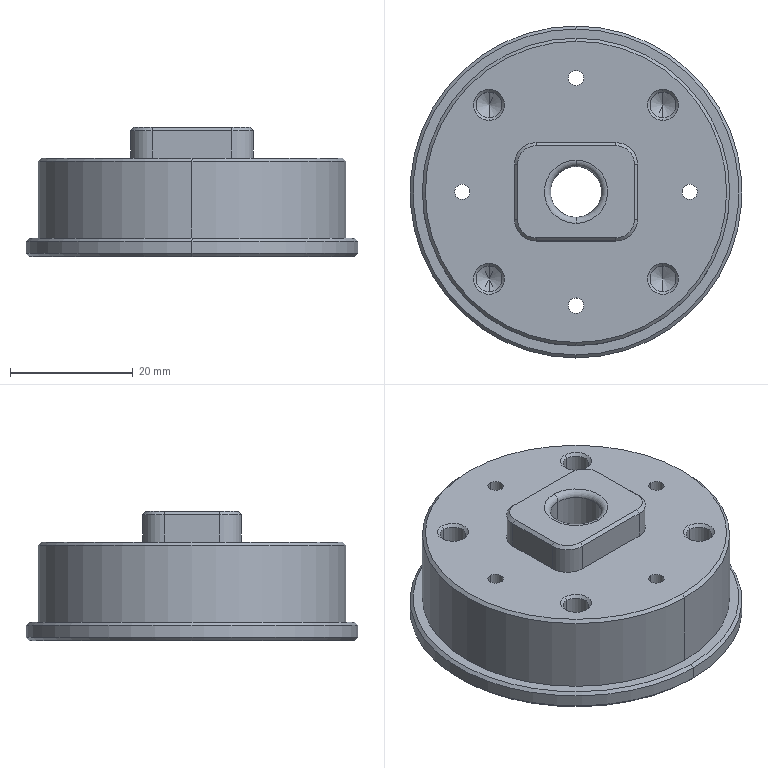NC program | NX | posted with a generic post | part box 54 x 54 x 21 mm
Lines 246 to 1139 of 9691:
(FLOOR_WALL_1_COPY_1 , TOOL : D4)
N478 T11 M6
N480 G54
N482 G17 G0 G90 X7.027 Y6.145 S9500 M3
N484 G43 Z30. H11
N486 Z1.5
N488 G94 G1 X7.252 Y5.92 Z1.483 F2200.
N490 X8.29 Y4.349 Z1.385
N492 X8.993 Y2.602 Z1.286
N494 X9.332 Y0.749 Z1.187
N496 Y-0.749 Z1.109
N498 X8.993 Y-2.602 Z1.01
N500 X8.29 Y-4.349 Z0.911
N502 X7.252 Y-5.92 Z0.813
N504 X5.92 Y-7.252 Z0.714
N506 X4.349 Y-8.29 Z0.615
N508 X2.602 Y-8.993 Z0.516
N510 X0.749 Y-9.332 Z0.418
N512 X-0.749 Z0.339
N514 X-2.602 Y-8.993 Z0.241
N516 X-4.349 Y-8.29 Z0.142
N518 X-5.92 Y-7.252 Z0.043
N520 X-7.252 Y-5.92 Z-0.056
N522 X-8.29 Y-4.349 Z-0.154
N524 X-8.993 Y-2.602 Z-0.253
N526 X-9.332 Y-0.749 Z-0.352
N528 Y0. Z-0.391
N530 G2 X0. Y9.332 R9.332
N532 X-9.332 Y0. R-9.332
N534 G1 X-9.9
N536 G3 X-9.895 Y-0.317 R9.9
N538 G2 X-11.188 Y-4.634 R7.1
N540 X-7.221 Y-6.773 R7.1
N542 G3 X-6.773 Y-7.221 R9.9
N544 G2 X-4.634 Y-11.188 R7.1
N546 X-0.317 Y-9.895 R7.1
N548 G3 X0.317 Y-9.895 R9.9
N550 G2 X4.634 Y-11.188 R7.1
N552 X6.773 Y-7.221 R7.1
N554 G3 X7.221 Y-6.773 R9.9
N556 G2 X11.188 Y-4.634 R7.1
N558 X9.895 Y-0.317 R7.1
N560 G3 X9.895 Y0.317 R9.9
N562 G2 X11.188 Y4.634 R7.1
N564 X7.221 Y6.773 R7.1
N566 G3 X6.773 Y7.221 R9.9
N568 G2 X4.634 Y11.188 R7.1
N570 X0.317 Y9.895 R7.1
N572 G3 X-0.317 Y9.895 R9.9
N574 G2 X-4.634 Y11.188 R7.1
N576 X-6.773 Y7.221 R7.1
N578 G3 X-7.221 Y6.773 R9.9
N580 G2 X-11.188 Y4.634 R7.1
N582 X-9.895 Y0.317 R7.1
N584 G3 X-9.9 Y0. R9.9
N586 G1 X-11.9
N588 G3 X-11.894 Y-0.381 R11.9
N590 G2 X-15.04 Y-5.255 R5.1
N592 G1 X-18.822 Y-6.822
N594 G3 X-19.309 Y-7.998 R0.9
N596 X-18.133 Y-8.485 R0.9
N598 G1 X-14.351 Y-6.918
N600 G2 X-8.679 Y-8.141 R5.1
N602 G3 X-8.141 Y-8.679 R11.9
N604 G2 X-6.918 Y-14.351 R5.1
N606 G1 X-8.485 Y-18.133
N608 G3 X-7.998 Y-19.309 R0.9
N610 X-6.822 Y-18.822 R0.9
N612 G1 X-5.255 Y-15.04
N614 G2 X-0.381 Y-11.894 R5.1
N616 G3 X0.381 Y-11.894 R11.9
N618 G2 X5.255 Y-15.04 R5.1
N620 G1 X6.822 Y-18.822
N622 G3 X7.998 Y-19.309 R0.9
N624 X8.485 Y-18.133 R0.9
N626 G1 X6.918 Y-14.351
N628 G2 X8.141 Y-8.679 R5.1
N630 G3 X8.679 Y-8.141 R11.9
N632 G2 X14.351 Y-6.918 R5.1
N634 G1 X18.133 Y-8.485
N636 G3 X19.309 Y-7.998 R0.9
N638 X18.822 Y-6.822 R0.9
N640 G1 X15.04 Y-5.255
N642 G2 X11.894 Y-0.381 R5.1
N644 G3 X11.894 Y0.381 R11.9
N646 G2 X15.04 Y5.255 R5.1
N648 G1 X18.822 Y6.822
N650 G3 X19.309 Y7.998 R0.9
N652 X18.133 Y8.485 R0.9
N654 G1 X14.351 Y6.918
N656 G2 X8.679 Y8.141 R5.1
N658 G3 X8.141 Y8.679 R11.9
N660 G2 X6.918 Y14.351 R5.1
N662 G1 X8.485 Y18.133
N664 G3 X7.998 Y19.309 R0.9
N666 X6.822 Y18.822 R0.9
N668 G1 X5.255 Y15.04
N670 G2 X0.381 Y11.894 R5.1
N672 G3 X-0.381 Y11.894 R11.9
N674 G2 X-5.255 Y15.04 R5.1
N676 G1 X-6.822 Y18.822
N678 G3 X-7.998 Y19.309 R0.9
N680 X-8.485 Y18.133 R0.9
N682 G1 X-6.918 Y14.351
N684 G2 X-8.141 Y8.679 R5.1
N686 G3 X-8.679 Y8.141 R11.9
N688 G2 X-14.351 Y6.918 R5.1
N690 G1 X-18.133 Y8.485
N692 G3 X-19.309 Y7.998 R0.9
N694 X-18.822 Y6.822 R0.9
N696 G1 X-15.04 Y5.255
N698 G2 X-11.894 Y0.381 R5.1
N700 G3 X-11.9 Y0. R11.9
N702 G1 Z1.109
N704 G0 Z30.
N706 X7.027 Y6.145
N708 Z1.109
N710 G1 X7.252 Y5.92 Z1.092
N712 X8.29 Y4.349 Z0.994
N714 X8.993 Y2.602 Z0.895
N716 X9.332 Y0.749 Z0.796
N718 Y-0.749 Z0.718
N720 X8.993 Y-2.602 Z0.619
N722 X8.29 Y-4.349 Z0.52
N724 X7.252 Y-5.92 Z0.422
N726 X5.92 Y-7.252 Z0.323
N728 X4.349 Y-8.29 Z0.224
N730 X2.602 Y-8.993 Z0.126
N732 X0.749 Y-9.332 Z0.027
N734 X-0.749 Z-0.052
N736 X-2.602 Y-8.993 Z-0.15
N738 X-4.349 Y-8.29 Z-0.249
N740 X-5.92 Y-7.252 Z-0.348
N742 X-7.252 Y-5.92 Z-0.446
N744 X-8.29 Y-4.349 Z-0.545
N746 X-8.993 Y-2.602 Z-0.644
N748 X-9.332 Y-0.749 Z-0.743
N750 Y0. Z-0.782
N752 G2 X0. Y9.332 R9.332
N754 X-9.332 Y0. R-9.332
N756 G1 X-9.9
N758 G3 X-9.895 Y-0.317 R9.9
N760 G2 X-11.188 Y-4.634 R7.1
N762 X-7.221 Y-6.773 R7.1
N764 G3 X-6.773 Y-7.221 R9.9
N766 G2 X-4.634 Y-11.188 R7.1
N768 X-0.317 Y-9.895 R7.1
N770 G3 X0.317 Y-9.895 R9.9
N772 G2 X4.634 Y-11.188 R7.1
N774 X6.773 Y-7.221 R7.1
N776 G3 X7.221 Y-6.773 R9.9
N778 G2 X11.188 Y-4.634 R7.1
N780 X9.895 Y-0.317 R7.1
N782 G3 X9.895 Y0.317 R9.9
N784 G2 X11.188 Y4.634 R7.1
N786 X7.221 Y6.773 R7.1
N788 G3 X6.773 Y7.221 R9.9
N790 G2 X4.634 Y11.188 R7.1
N792 X0.317 Y9.895 R7.1
N794 G3 X-0.317 Y9.895 R9.9
N796 G2 X-4.634 Y11.188 R7.1
N798 X-6.773 Y7.221 R7.1
N800 G3 X-7.221 Y6.773 R9.9
N802 G2 X-11.188 Y4.634 R7.1
N804 X-9.895 Y0.317 R7.1
N806 G3 X-9.9 Y0. R9.9
N808 G1 X-11.9
N810 G3 X-11.894 Y-0.381 R11.9
N812 G2 X-15.04 Y-5.255 R5.1
N814 G1 X-18.822 Y-6.822
N816 G3 X-19.309 Y-7.998 R0.9
N818 X-18.133 Y-8.485 R0.9
N820 G1 X-14.351 Y-6.918
N822 G2 X-8.679 Y-8.141 R5.1
N824 G3 X-8.141 Y-8.679 R11.9
N826 G2 X-6.918 Y-14.351 R5.1
N828 G1 X-8.485 Y-18.133
N830 G3 X-7.998 Y-19.309 R0.9
N832 X-6.822 Y-18.822 R0.9
N834 G1 X-5.255 Y-15.04
N836 G2 X-0.381 Y-11.894 R5.1
N838 G3 X0.381 Y-11.894 R11.9
N840 G2 X5.255 Y-15.04 R5.1
N842 G1 X6.822 Y-18.822
N844 G3 X7.998 Y-19.309 R0.9
N846 X8.485 Y-18.133 R0.9
N848 G1 X6.918 Y-14.351
N850 G2 X8.141 Y-8.679 R5.1
N852 G3 X8.679 Y-8.141 R11.9
N854 G2 X14.351 Y-6.918 R5.1
N856 G1 X18.133 Y-8.485
N858 G3 X19.309 Y-7.998 R0.9
N860 X18.822 Y-6.822 R0.9
N862 G1 X15.04 Y-5.255
N864 G2 X11.894 Y-0.381 R5.1
N866 G3 X11.894 Y0.381 R11.9
N868 G2 X15.04 Y5.255 R5.1
N870 G1 X18.822 Y6.822
N872 G3 X19.309 Y7.998 R0.9
N874 X18.133 Y8.485 R0.9
N876 G1 X14.351 Y6.918
N878 G2 X8.679 Y8.141 R5.1
N880 G3 X8.141 Y8.679 R11.9
N882 G2 X6.918 Y14.351 R5.1
N884 G1 X8.485 Y18.133
N886 G3 X7.998 Y19.309 R0.9
N888 X6.822 Y18.822 R0.9
N890 G1 X5.255 Y15.04
N892 G2 X0.381 Y11.894 R5.1
N894 G3 X-0.381 Y11.894 R11.9
N896 G2 X-5.255 Y15.04 R5.1
N898 G1 X-6.822 Y18.822
N900 G3 X-7.998 Y19.309 R0.9
N902 X-8.485 Y18.133 R0.9
N904 G1 X-6.918 Y14.351
N906 G2 X-8.141 Y8.679 R5.1
N908 G3 X-8.679 Y8.141 R11.9
N910 G2 X-14.351 Y6.918 R5.1
N912 G1 X-18.133 Y8.485
N914 G3 X-19.309 Y7.998 R0.9
N916 X-18.822 Y6.822 R0.9
N918 G1 X-15.04 Y5.255
N920 G2 X-11.894 Y0.381 R5.1
N922 G3 X-11.9 Y0. R11.9
N924 G1 Z0.718
N926 G0 Z30.
N928 X7.027 Y6.145
N930 Z0.718
N932 G1 X7.252 Y5.92 Z0.702
N934 X8.29 Y4.349 Z0.603
N936 X8.993 Y2.602 Z0.504
N938 X9.332 Y0.749 Z0.405
N940 Y-0.749 Z0.327
N942 X8.993 Y-2.602 Z0.228
N944 X8.29 Y-4.349 Z0.129
N946 X7.252 Y-5.92 Z0.031
N948 X5.92 Y-7.252 Z-0.068
N950 X4.349 Y-8.29 Z-0.167
N952 X2.602 Y-8.993 Z-0.265
N954 X0.749 Y-9.332 Z-0.364
N956 X-0.749 Z-0.443
N958 X-2.602 Y-8.993 Z-0.541
N960 X-4.349 Y-8.29 Z-0.64
N962 X-5.92 Y-7.252 Z-0.739
N964 X-7.252 Y-5.92 Z-0.837
N966 X-8.29 Y-4.349 Z-0.936
N968 X-8.993 Y-2.602 Z-1.035
N970 X-9.332 Y-0.749 Z-1.133
N972 Y0. Z-1.173
N974 G2 X0. Y9.332 R9.332
N976 X-9.332 Y0. R-9.332
N978 G1 X-9.9
N980 G3 X-9.895 Y-0.317 R9.9
N982 G2 X-11.188 Y-4.634 R7.1
N984 X-7.221 Y-6.773 R7.1
N986 G3 X-6.773 Y-7.221 R9.9
N988 G2 X-4.634 Y-11.188 R7.1
N990 X-0.317 Y-9.895 R7.1
N992 G3 X0.317 Y-9.895 R9.9
N994 G2 X4.634 Y-11.188 R7.1
N996 X6.773 Y-7.221 R7.1
N998 G3 X7.221 Y-6.773 R9.9
N1000 G2 X11.188 Y-4.634 R7.1
N1002 X9.895 Y-0.317 R7.1
N1004 G3 X9.895 Y0.317 R9.9
N1006 G2 X11.188 Y4.634 R7.1
N1008 X7.221 Y6.773 R7.1
N1010 G3 X6.773 Y7.221 R9.9
N1012 G2 X4.634 Y11.188 R7.1
N1014 X0.317 Y9.895 R7.1
N1016 G3 X-0.317 Y9.895 R9.9
N1018 G2 X-4.634 Y11.188 R7.1
N1020 X-6.773 Y7.221 R7.1
N1022 G3 X-7.221 Y6.773 R9.9
N1024 G2 X-11.188 Y4.634 R7.1
N1026 X-9.895 Y0.317 R7.1
N1028 G3 X-9.9 Y0. R9.9
N1030 G1 X-11.9
N1032 G3 X-11.894 Y-0.381 R11.9
N1034 G2 X-15.04 Y-5.255 R5.1
N1036 G1 X-18.822 Y-6.822
N1038 G3 X-19.309 Y-7.998 R0.9
N1040 X-18.133 Y-8.485 R0.9
N1042 G1 X-14.351 Y-6.918
N1044 G2 X-8.679 Y-8.141 R5.1
N1046 G3 X-8.141 Y-8.679 R11.9
N1048 G2 X-6.918 Y-14.351 R5.1
N1050 G1 X-8.485 Y-18.133
N1052 G3 X-7.998 Y-19.309 R0.9
N1054 X-6.822 Y-18.822 R0.9
N1056 G1 X-5.255 Y-15.04
N1058 G2 X-0.381 Y-11.894 R5.1
N1060 G3 X0.381 Y-11.894 R11.9
N1062 G2 X5.255 Y-15.04 R5.1
N1064 G1 X6.822 Y-18.822
N1066 G3 X7.998 Y-19.309 R0.9
N1068 X8.485 Y-18.133 R0.9
N1070 G1 X6.918 Y-14.351
N1072 G2 X8.141 Y-8.679 R5.1
N1074 G3 X8.679 Y-8.141 R11.9
N1076 G2 X14.351 Y-6.918 R5.1
N1078 G1 X18.133 Y-8.485
N1080 G3 X19.309 Y-7.998 R0.9
N1082 X18.822 Y-6.822 R0.9
N1084 G1 X15.04 Y-5.255
N1086 G2 X11.894 Y-0.381 R5.1
N1088 G3 X11.894 Y0.381 R11.9
N1090 G2 X15.04 Y5.255 R5.1
N1092 G1 X18.822 Y6.822
N1094 G3 X19.309 Y7.998 R0.9
N1096 X18.133 Y8.485 R0.9
N1098 G1 X14.351 Y6.918
N1100 G2 X8.679 Y8.141 R5.1
N1102 G3 X8.141 Y8.679 R11.9
N1104 G2 X6.918 Y14.351 R5.1
N1106 G1 X8.485 Y18.133
N1108 G3 X7.998 Y19.309 R0.9
N1110 X6.822 Y18.822 R0.9
N1112 G1 X5.255 Y15.04
N1114 G2 X0.381 Y11.894 R5.1
N1116 G3 X-0.381 Y11.894 R11.9
N1118 G2 X-5.255 Y15.04 R5.1
N1120 G1 X-6.822 Y18.822
N1122 G3 X-7.998 Y19.309 R0.9
N1124 X-8.485 Y18.133 R0.9
N1126 G1 X-6.918 Y14.351
N1128 G2 X-8.141 Y8.679 R5.1
N1130 G3 X-8.679 Y8.141 R11.9
N1132 G2 X-14.351 Y6.918 R5.1
N1134 G1 X-18.133 Y8.485
N1136 G3 X-19.309 Y7.998 R0.9
N1138 X-18.822 Y6.822 R0.9
N1140 G1 X-15.04 Y5.255
N1142 G2 X-11.894 Y0.381 R5.1
N1144 G3 X-11.9 Y0. R11.9
N1146 G1 Z0.327
N1148 G0 Z30.
N1150 X7.027 Y6.145
N1152 Z0.327
N1154 G1 X7.252 Y5.92 Z0.311
N1156 X8.29 Y4.349 Z0.212
N1158 X8.993 Y2.602 Z0.113
N1160 X9.332 Y0.749 Z0.014
N1162 Y-0.749 Z-0.064
N1164 X8.993 Y-2.602 Z-0.163
N1166 X8.29 Y-4.349 Z-0.261
N1168 X7.252 Y-5.92 Z-0.36
N1170 X5.92 Y-7.252 Z-0.459
N1172 X4.349 Y-8.29 Z-0.558
N1174 X2.602 Y-8.993 Z-0.656
N1176 X0.749 Y-9.332 Z-0.755
N1178 X-0.749 Z-0.833
N1180 X-2.602 Y-8.993 Z-0.932
N1182 X-4.349 Y-8.29 Z-1.031
N1184 X-5.92 Y-7.252 Z-1.13
N1186 X-7.252 Y-5.92 Z-1.228
N1188 X-8.29 Y-4.349 Z-1.327
N1190 X-8.993 Y-2.602 Z-1.426
N1192 X-9.332 Y-0.749 Z-1.524
N1194 Y0. Z-1.564
N1196 G2 X0. Y9.332 R9.332
N1198 X-9.332 Y0. R-9.332
N1200 G1 X-9.9
N1202 G3 X-9.895 Y-0.317 R9.9
N1204 G2 X-11.188 Y-4.634 R7.1
N1206 X-7.221 Y-6.773 R7.1
N1208 G3 X-6.773 Y-7.221 R9.9
N1210 G2 X-4.634 Y-11.188 R7.1
N1212 X-0.317 Y-9.895 R7.1
N1214 G3 X0.317 Y-9.895 R9.9
N1216 G2 X4.634 Y-11.188 R7.1
N1218 X6.773 Y-7.221 R7.1
N1220 G3 X7.221 Y-6.773 R9.9
N1222 G2 X11.188 Y-4.634 R7.1
N1224 X9.895 Y-0.317 R7.1
N1226 G3 X9.895 Y0.317 R9.9
N1228 G2 X11.188 Y4.634 R7.1
N1230 X7.221 Y6.773 R7.1
N1232 G3 X6.773 Y7.221 R9.9
N1234 G2 X4.634 Y11.188 R7.1
N1236 X0.317 Y9.895 R7.1
N1238 G3 X-0.317 Y9.895 R9.9
N1240 G2 X-4.634 Y11.188 R7.1
N1242 X-6.773 Y7.221 R7.1
N1244 G3 X-7.221 Y6.773 R9.9
N1246 G2 X-11.188 Y4.634 R7.1
N1248 X-9.895 Y0.317 R7.1
N1250 G3 X-9.9 Y0. R9.9
N1252 G1 X-11.9
N1254 G3 X-11.894 Y-0.381 R11.9
N1256 G2 X-15.04 Y-5.255 R5.1
N1258 G1 X-18.822 Y-6.822
N1260 G3 X-19.309 Y-7.998 R0.9
N1262 X-18.133 Y-8.485 R0.9
N1264 G1 X-14.351 Y-6.918
N1266 G2 X-8.679 Y-8.141 R5.1
N1268 G3 X-8.141 Y-8.679 R11.9
N1270 G2 X-6.918 Y-14.351 R5.1
N1272 G1 X-8.485 Y-18.133
N1274 G3 X-7.998 Y-19.309 R0.9
N1276 X-6.822 Y-18.822 R0.9
N1278 G1 X-5.255 Y-15.04
N1280 G2 X-0.381 Y-11.894 R5.1
N1282 G3 X0.381 Y-11.894 R11.9
N1284 G2 X5.255 Y-15.04 R5.1
N1286 G1 X6.822 Y-18.822
N1288 G3 X7.998 Y-19.309 R0.9
N1290 X8.485 Y-18.133 R0.9
N1292 G1 X6.918 Y-14.351
N1294 G2 X8.141 Y-8.679 R5.1
N1296 G3 X8.679 Y-8.141 R11.9
N1298 G2 X14.351 Y-6.918 R5.1
N1300 G1 X18.133 Y-8.485
N1302 G3 X19.309 Y-7.998 R0.9
N1304 X18.822 Y-6.822 R0.9
N1306 G1 X15.04 Y-5.255
N1308 G2 X11.894 Y-0.381 R5.1
N1310 G3 X11.894 Y0.381 R11.9
N1312 G2 X15.04 Y5.255 R5.1
N1314 G1 X18.822 Y6.822
N1316 G3 X19.309 Y7.998 R0.9
N1318 X18.133 Y8.485 R0.9
N1320 G1 X14.351 Y6.918
N1322 G2 X8.679 Y8.141 R5.1
N1324 G3 X8.141 Y8.679 R11.9
N1326 G2 X6.918 Y14.351 R5.1
N1328 G1 X8.485 Y18.133
N1330 G3 X7.998 Y19.309 R0.9
N1332 X6.822 Y18.822 R0.9
N1334 G1 X5.255 Y15.04
N1336 G2 X0.381 Y11.894 R5.1
N1338 G3 X-0.381 Y11.894 R11.9
N1340 G2 X-5.255 Y15.04 R5.1
N1342 G1 X-6.822 Y18.822
N1344 G3 X-7.998 Y19.309 R0.9
N1346 X-8.485 Y18.133 R0.9
N1348 G1 X-6.918 Y14.351
N1350 G2 X-8.141 Y8.679 R5.1
N1352 G3 X-8.679 Y8.141 R11.9
N1354 G2 X-14.351 Y6.918 R5.1
N1356 G1 X-18.133 Y8.485
N1358 G3 X-19.309 Y7.998 R0.9
N1360 X-18.822 Y6.822 R0.9
N1362 G1 X-15.04 Y5.255
N1364 G2 X-11.894 Y0.381 R5.1
N1366 G3 X-11.9 Y0. R11.9
N1368 G1 Z-0.064
N1370 G0 Z30.
N1372 X7.027 Y6.145
N1374 Z-0.064
N1376 G1 X7.252 Y5.92 Z-0.08
N1378 X8.29 Y4.349 Z-0.179
N1380 X8.993 Y2.602 Z-0.278
N1382 X9.332 Y0.749 Z-0.376
N1384 Y-0.749 Z-0.455
N1386 X8.993 Y-2.602 Z-0.554
N1388 X8.29 Y-4.349 Z-0.652
N1390 X7.252 Y-5.92 Z-0.751
N1392 X5.92 Y-7.252 Z-0.85
N1394 X4.349 Y-8.29 Z-0.948
N1396 X2.602 Y-8.993 Z-1.047
N1398 X0.749 Y-9.332 Z-1.146
N1400 X-0.749 Z-1.224
N1402 X-2.602 Y-8.993 Z-1.323
N1404 X-4.349 Y-8.29 Z-1.422
N1406 X-5.92 Y-7.252 Z-1.52
N1408 X-7.252 Y-5.92 Z-1.619
N1410 X-8.29 Y-4.349 Z-1.718
N1412 X-8.993 Y-2.602 Z-1.817
N1414 X-9.332 Y-0.749 Z-1.915
N1416 Y0. Z-1.955
N1418 G2 X0. Y9.332 R9.332
N1420 X-9.332 Y0. R-9.332
N1422 G1 X-9.9
N1424 G3 X-9.895 Y-0.317 R9.9
N1426 G2 X-11.188 Y-4.634 R7.1
N1428 X-7.221 Y-6.773 R7.1
N1430 G3 X-6.773 Y-7.221 R9.9
N1432 G2 X-4.634 Y-11.188 R7.1
N1434 X-0.317 Y-9.895 R7.1
N1436 G3 X0.317 Y-9.895 R9.9
N1438 G2 X4.634 Y-11.188 R7.1
N1440 X6.773 Y-7.221 R7.1
N1442 G3 X7.221 Y-6.773 R9.9
N1444 G2 X11.188 Y-4.634 R7.1
N1446 X9.895 Y-0.317 R7.1
N1448 G3 X9.895 Y0.317 R9.9
N1450 G2 X11.188 Y4.634 R7.1
N1452 X7.221 Y6.773 R7.1
N1454 G3 X6.773 Y7.221 R9.9
N1456 G2 X4.634 Y11.188 R7.1
N1458 X0.317 Y9.895 R7.1
N1460 G3 X-0.317 Y9.895 R9.9
N1462 G2 X-4.634 Y11.188 R7.1
N1464 X-6.773 Y7.221 R7.1
N1466 G3 X-7.221 Y6.773 R9.9
N1468 G2 X-11.188 Y4.634 R7.1
N1470 X-9.895 Y0.317 R7.1
N1472 G3 X-9.9 Y0. R9.9
N1474 G1 X-11.9
N1476 G3 X-11.894 Y-0.381 R11.9
N1478 G2 X-15.04 Y-5.255 R5.1
N1480 G1 X-18.822 Y-6.822
N1482 G3 X-19.309 Y-7.998 R0.9
N1484 X-18.133 Y-8.485 R0.9
N1486 G1 X-14.351 Y-6.918
N1488 G2 X-8.679 Y-8.141 R5.1
N1490 G3 X-8.141 Y-8.679 R11.9
N1492 G2 X-6.918 Y-14.351 R5.1
N1494 G1 X-8.485 Y-18.133
N1496 G3 X-7.998 Y-19.309 R0.9
N1498 X-6.822 Y-18.822 R0.9
N1500 G1 X-5.255 Y-15.04
N1502 G2 X-0.381 Y-11.894 R5.1
N1504 G3 X0.381 Y-11.894 R11.9
N1506 G2 X5.255 Y-15.04 R5.1
N1508 G1 X6.822 Y-18.822
N1510 G3 X7.998 Y-19.309 R0.9
N1512 X8.485 Y-18.133 R0.9
N1514 G1 X6.918 Y-14.351
N1516 G2 X8.141 Y-8.679 R5.1
N1518 G3 X8.679 Y-8.141 R11.9
N1520 G2 X14.351 Y-6.918 R5.1
N1522 G1 X18.133 Y-8.485
N1524 G3 X19.309 Y-7.998 R0.9
N1526 X18.822 Y-6.822 R0.9
N1528 G1 X15.04 Y-5.255
N1530 G2 X11.894 Y-0.381 R5.1
N1532 G3 X11.894 Y0.381 R11.9
N1534 G2 X15.04 Y5.255 R5.1
N1536 G1 X18.822 Y6.822
N1538 G3 X19.309 Y7.998 R0.9
N1540 X18.133 Y8.485 R0.9
N1542 G1 X14.351 Y6.918
N1544 G2 X8.679 Y8.141 R5.1
N1546 G3 X8.141 Y8.679 R11.9
N1548 G2 X6.918 Y14.351 R5.1
N1550 G1 X8.485 Y18.133
N1552 G3 X7.998 Y19.309 R0.9
N1554 X6.822 Y18.822 R0.9
N1556 G1 X5.255 Y15.04
N1558 G2 X0.381 Y11.894 R5.1
N1560 G3 X-0.381 Y11.894 R11.9
N1562 G2 X-5.255 Y15.04 R5.1
N1564 G1 X-6.822 Y18.822
N1566 G3 X-7.998 Y19.309 R0.9
N1568 X-8.485 Y18.133 R0.9
N1570 G1 X-6.918 Y14.351
N1572 G2 X-8.141 Y8.679 R5.1
N1574 G3 X-8.679 Y8.141 R11.9
N1576 G2 X-14.351 Y6.918 R5.1
N1578 G1 X-18.133 Y8.485
N1580 G3 X-19.309 Y7.998 R0.9
N1582 X-18.822 Y6.822 R0.9
N1584 G1 X-15.04 Y5.255
N1586 G2 X-11.894 Y0.381 R5.1
N1588 G3 X-11.9 Y0. R11.9
N1590 G1 Z-0.455
N1592 G0 Z30.
N1594 X7.027 Y6.145
N1596 Z-0.455
N1598 G1 X7.252 Y5.92 Z-0.471
N1600 X8.29 Y4.349 Z-0.57
N1602 X8.993 Y2.602 Z-0.669
N1604 X9.332 Y0.749 Z-0.767
N1606 Y-0.749 Z-0.846
N1608 X8.993 Y-2.602 Z-0.945
N1610 X8.29 Y-4.349 Z-1.043
N1612 X7.252 Y-5.92 Z-1.142
N1614 X5.92 Y-7.252 Z-1.241
N1616 X4.349 Y-8.29 Z-1.339
N1618 X2.602 Y-8.993 Z-1.438
N1620 X0.749 Y-9.332 Z-1.537
N1622 X-0.749 Z-1.615
N1624 X-2.602 Y-8.993 Z-1.714
N1626 X-4.349 Y-8.29 Z-1.813
N1628 X-5.92 Y-7.252 Z-1.911
N1630 X-7.252 Y-5.92 Z-2.01
N1632 X-8.29 Y-4.349 Z-2.109
N1634 X-8.993 Y-2.602 Z-2.208
N1636 X-9.332 Y-0.749 Z-2.306
N1638 Y0. Z-2.345
N1640 G2 X0. Y9.332 R9.332
N1642 X-9.332 Y0. R-9.332
N1644 G1 X-9.9
N1646 G3 X-9.895 Y-0.317 R9.9
N1648 G2 X-11.188 Y-4.634 R7.1
N1650 X-7.221 Y-6.773 R7.1
N1652 G3 X-6.773 Y-7.221 R9.9
N1654 G2 X-4.634 Y-11.188 R7.1
N1656 X-0.317 Y-9.895 R7.1
N1658 G3 X0.317 Y-9.895 R9.9
N1660 G2 X4.634 Y-11.188 R7.1
N1662 X6.773 Y-7.221 R7.1
N1664 G3 X7.221 Y-6.773 R9.9
N1666 G2 X11.188 Y-4.634 R7.1
N1668 X9.895 Y-0.317 R7.1
N1670 G3 X9.895 Y0.317 R9.9
N1672 G2 X11.188 Y4.634 R7.1
N1674 X7.221 Y6.773 R7.1
N1676 G3 X6.773 Y7.221 R9.9
N1678 G2 X4.634 Y11.188 R7.1
N1680 X0.317 Y9.895 R7.1
N1682 G3 X-0.317 Y9.895 R9.9
N1684 G2 X-4.634 Y11.188 R7.1
N1686 X-6.773 Y7.221 R7.1
N1688 G3 X-7.221 Y6.773 R9.9
N1690 G2 X-11.188 Y4.634 R7.1
N1692 X-9.895 Y0.317 R7.1
N1694 G3 X-9.9 Y0. R9.9
N1696 G1 X-11.9
N1698 G3 X-11.894 Y-0.381 R11.9
N1700 G2 X-15.04 Y-5.255 R5.1
N1702 G1 X-18.822 Y-6.822
N1704 G3 X-19.309 Y-7.998 R0.9
N1706 X-18.133 Y-8.485 R0.9
N1708 G1 X-14.351 Y-6.918
N1710 G2 X-8.679 Y-8.141 R5.1
N1712 G3 X-8.141 Y-8.679 R11.9
N1714 G2 X-6.918 Y-14.351 R5.1
N1716 G1 X-8.485 Y-18.133
N1718 G3 X-7.998 Y-19.309 R0.9
N1720 X-6.822 Y-18.822 R0.9
N1722 G1 X-5.255 Y-15.04
N1724 G2 X-0.381 Y-11.894 R5.1
N1726 G3 X0.381 Y-11.894 R11.9
N1728 G2 X5.255 Y-15.04 R5.1
N1730 G1 X6.822 Y-18.822
N1732 G3 X7.998 Y-19.309 R0.9
N1734 X8.485 Y-18.133 R0.9
N1736 G1 X6.918 Y-14.351
N1738 G2 X8.141 Y-8.679 R5.1
N1740 G3 X8.679 Y-8.141 R11.9
N1742 G2 X14.351 Y-6.918 R5.1
N1744 G1 X18.133 Y-8.485
N1746 G3 X19.309 Y-7.998 R0.9
N1748 X18.822 Y-6.822 R0.9
N1750 G1 X15.04 Y-5.255
N1752 G2 X11.894 Y-0.381 R5.1
N1754 G3 X11.894 Y0.381 R11.9
N1756 G2 X15.04 Y5.255 R5.1
N1758 G1 X18.822 Y6.822
N1760 G3 X19.309 Y7.998 R0.9
N1762 X18.133 Y8.485 R0.9
N1764 G1 X14.351 Y6.918
N1766 G2 X8.679 Y8.141 R5.1
N1768 G3 X8.141 Y8.679 R11.9
N1770 G2 X6.918 Y14.351 R5.1
N1772 G1 X8.485 Y18.133
N1774 G3 X7.998 Y19.309 R0.9
N1776 X6.822 Y18.822 R0.9
N1778 G1 X5.255 Y15.04
N1780 G2 X0.381 Y11.894 R5.1
N1782 G3 X-0.381 Y11.894 R11.9
N1784 G2 X-5.255 Y15.04 R5.1
N1786 G1 X-6.822 Y18.822
N1788 G3 X-7.998 Y19.309 R0.9
N1790 X-8.485 Y18.133 R0.9
N1792 G1 X-6.918 Y14.351
N1794 G2 X-8.141 Y8.679 R5.1
N1796 G3 X-8.679 Y8.141 R11.9
N1798 G2 X-14.351 Y6.918 R5.1
N1800 G1 X-18.133 Y8.485
N1802 G3 X-19.309 Y7.998 R0.9
N1804 X-18.822 Y6.822 R0.9
N1806 G1 X-15.04 Y5.255
N1808 G2 X-11.894 Y0.381 R5.1
N1810 G3 X-11.9 Y0. R11.9
N1812 G1 Z-0.845
N1814 G0 Z30.
N1816 X7.027 Y6.145
N1818 Z-0.845
N1820 G1 X7.252 Y5.92 Z-0.862
N1822 X8.29 Y4.349 Z-0.961
N1824 X8.993 Y2.602 Z-1.06
N1826 X9.332 Y0.749 Z-1.158
N1828 Y-0.749 Z-1.237
N1830 X8.993 Y-2.602 Z-1.335
N1832 X8.29 Y-4.349 Z-1.434
N1834 X7.252 Y-5.92 Z-1.533
N1836 X5.92 Y-7.252 Z-1.632
N1838 X4.349 Y-8.29 Z-1.73
N1840 X2.602 Y-8.993 Z-1.829
N1842 X0.749 Y-9.332 Z-1.928
N1844 X-0.749 Z-2.006
N1846 X-2.602 Y-8.993 Z-2.105
N1848 X-4.349 Y-8.29 Z-2.204
N1850 X-5.92 Y-7.252 Z-2.302
N1852 X-7.252 Y-5.92 Z-2.401
N1854 X-8.29 Y-4.349 Z-2.5
N1856 X-8.993 Y-2.602 Z-2.598
N1858 X-9.332 Y-0.749 Z-2.697
N1860 Y0. Z-2.736
N1862 G2 X0. Y9.332 R9.332
N1864 X-9.332 Y0. R-9.332
N1866 G1 X-9.9
N1868 G3 X-9.895 Y-0.317 R9.9
N1870 G2 X-11.188 Y-4.634 R7.1
N1872 X-7.221 Y-6.773 R7.1
N1874 G3 X-6.773 Y-7.221 R9.9
N1876 G2 X-4.634 Y-11.188 R7.1
N1878 X-0.317 Y-9.895 R7.1
N1880 G3 X0.317 Y-9.895 R9.9
N1882 G2 X4.634 Y-11.188 R7.1
N1884 X6.773 Y-7.221 R7.1
N1886 G3 X7.221 Y-6.773 R9.9
N1888 G2 X11.188 Y-4.634 R7.1
N1890 X9.895 Y-0.317 R7.1
N1892 G3 X9.895 Y0.317 R9.9
N1894 G2 X11.188 Y4.634 R7.1
N1896 X7.221 Y6.773 R7.1
N1898 G3 X6.773 Y7.221 R9.9
N1900 G2 X4.634 Y11.188 R7.1
N1902 X0.317 Y9.895 R7.1
N1904 G3 X-0.317 Y9.895 R9.9
N1906 G2 X-4.634 Y11.188 R7.1
N1908 X-6.773 Y7.221 R7.1
N1910 G3 X-7.221 Y6.773 R9.9
N1912 G2 X-11.188 Y4.634 R7.1
N1914 X-9.895 Y0.317 R7.1
N1916 G3 X-9.9 Y0. R9.9
N1918 G1 X-11.9
N1920 G3 X-11.894 Y-0.381 R11.9
N1922 G2 X-15.04 Y-5.255 R5.1
N1924 G1 X-18.822 Y-6.822
N1926 G3 X-19.309 Y-7.998 R0.9
N1928 X-18.133 Y-8.485 R0.9
N1930 G1 X-14.351 Y-6.918
N1932 G2 X-8.679 Y-8.141 R5.1
N1934 G3 X-8.141 Y-8.679 R11.9
N1936 G2 X-6.918 Y-14.351 R5.1
N1938 G1 X-8.485 Y-18.133
N1940 G3 X-7.998 Y-19.309 R0.9
N1942 X-6.822 Y-18.822 R0.9
N1944 G1 X-5.255 Y-15.04
N1946 G2 X-0.381 Y-11.894 R5.1
N1948 G3 X0.381 Y-11.894 R11.9
N1950 G2 X5.255 Y-15.04 R5.1
N1952 G1 X6.822 Y-18.822
N1954 G3 X7.998 Y-19.309 R0.9
N1956 X8.485 Y-18.133 R0.9
N1958 G1 X6.918 Y-14.351
N1960 G2 X8.141 Y-8.679 R5.1
N1962 G3 X8.679 Y-8.141 R11.9
N1964 G2 X14.351 Y-6.918 R5.1
N1966 G1 X18.133 Y-8.485
N1968 G3 X19.309 Y-7.998 R0.9
N1970 X18.822 Y-6.822 R0.9
N1972 G1 X15.04 Y-5.255
N1974 G2 X11.894 Y-0.381 R5.1
N1976 G3 X11.894 Y0.381 R11.9
N1978 G2 X15.04 Y5.255 R5.1
N1980 G1 X18.822 Y6.822
N1982 G3 X19.309 Y7.998 R0.9
N1984 X18.133 Y8.485 R0.9
N1986 G1 X14.351 Y6.918
N1988 G2 X8.679 Y8.141 R5.1
N1990 G3 X8.141 Y8.679 R11.9
N1992 G2 X6.918 Y14.351 R5.1
N1994 G1 X8.485 Y18.133
N1996 G3 X7.998 Y19.309 R0.9
N1998 X6.822 Y18.822 R0.9
N2000 G1 X5.255 Y15.04
N2002 G2 X0.381 Y11.894 R5.1
N2004 G3 X-0.381 Y11.894 R11.9
N2006 G2 X-5.255 Y15.04 R5.1
N2008 G1 X-6.822 Y18.822
N2010 G3 X-7.998 Y19.309 R0.9
N2012 X-8.485 Y18.133 R0.9
N2014 G1 X-6.918 Y14.351
N2016 G2 X-8.141 Y8.679 R5.1
N2018 G3 X-8.679 Y8.141 R11.9
N2020 G2 X-14.351 Y6.918 R5.1
N2022 G1 X-18.133 Y8.485
N2024 G3 X-19.309 Y7.998 R0.9
N2026 X-18.822 Y6.822 R0.9
N2028 G1 X-15.04 Y5.255
N2030 G2 X-11.894 Y0.381 R5.1
N2032 G3 X-11.9 Y0. R11.9
N2034 G1 Z-1.236
N2036 G0 Z30.
N2038 X7.027 Y6.145
N2040 Z-1.236
N2042 G1 X7.252 Y5.92 Z-1.253
N2044 X8.29 Y4.349 Z-1.352
N2046 X8.993 Y2.602 Z-1.45
N2048 X9.332 Y0.749 Z-1.549
N2050 Y-0.749 Z-1.628
N2052 X8.993 Y-2.602 Z-1.726
N2054 X8.29 Y-4.349 Z-1.825
N2056 X7.252 Y-5.92 Z-1.924
N2058 X5.92 Y-7.252 Z-2.022
N2060 X4.349 Y-8.29 Z-2.121
N2062 X2.602 Y-8.993 Z-2.22
N2064 X0.749 Y-9.332 Z-2.319
N2066 X-0.749 Z-2.397
N2068 X-2.602 Y-8.993 Z-2.496
N2070 X-4.349 Y-8.29 Z-2.594
N2072 X-5.92 Y-7.252 Z-2.693
N2074 X-7.252 Y-5.92 Z-2.792
N2076 X-8.29 Y-4.349 Z-2.891
N2078 X-8.993 Y-2.602 Z-2.989
N2080 X-9.332 Y-0.749 Z-3.088
N2082 Y0. Z-3.127
N2084 G2 X0. Y9.332 R9.332
N2086 X-9.332 Y0. R-9.332
N2088 G1 X-9.9
N2090 G3 X-9.895 Y-0.317 R9.9
N2092 G2 X-11.188 Y-4.634 R7.1
N2094 X-7.221 Y-6.773 R7.1
N2096 G3 X-6.773 Y-7.221 R9.9
N2098 G2 X-4.634 Y-11.188 R7.1
N2100 X-0.317 Y-9.895 R7.1
N2102 G3 X0.317 Y-9.895 R9.9
N2104 G2 X4.634 Y-11.188 R7.1
N2106 X6.773 Y-7.221 R7.1
N2108 G3 X7.221 Y-6.773 R9.9
N2110 G2 X11.188 Y-4.634 R7.1
N2112 X9.895 Y-0.317 R7.1
N2114 G3 X9.895 Y0.317 R9.9
N2116 G2 X11.188 Y4.634 R7.1
N2118 X7.221 Y6.773 R7.1
N2120 G3 X6.773 Y7.221 R9.9
N2122 G2 X4.634 Y11.188 R7.1
N2124 X0.317 Y9.895 R7.1
N2126 G3 X-0.317 Y9.895 R9.9
N2128 G2 X-4.634 Y11.188 R7.1
N2130 X-6.773 Y7.221 R7.1
N2132 G3 X-7.221 Y6.773 R9.9
N2134 G2 X-11.188 Y4.634 R7.1
N2136 X-9.895 Y0.317 R7.1
N2138 G3 X-9.9 Y0. R9.9
N2140 G1 X-11.9
N2142 G3 X-11.894 Y-0.381 R11.9
N2144 G2 X-15.04 Y-5.255 R5.1
N2146 G1 X-18.822 Y-6.822
N2148 G3 X-19.309 Y-7.998 R0.9
N2150 X-18.133 Y-8.485 R0.9
N2152 G1 X-14.351 Y-6.918
N2154 G2 X-8.679 Y-8.141 R5.1
N2156 G3 X-8.141 Y-8.679 R11.9
N2158 G2 X-6.918 Y-14.351 R5.1
N2160 G1 X-8.485 Y-18.133
N2162 G3 X-7.998 Y-19.309 R0.9
N2164 X-6.822 Y-18.822 R0.9
N2166 G1 X-5.255 Y-15.04
N2168 G2 X-0.381 Y-11.894 R5.1
N2170 G3 X0.381 Y-11.894 R11.9
N2172 G2 X5.255 Y-15.04 R5.1
N2174 G1 X6.822 Y-18.822
N2176 G3 X7.998 Y-19.309 R0.9
N2178 X8.485 Y-18.133 R0.9
N2180 G1 X6.918 Y-14.351
N2182 G2 X8.141 Y-8.679 R5.1
N2184 G3 X8.679 Y-8.141 R11.9
N2186 G2 X14.351 Y-6.918 R5.1
N2188 G1 X18.133 Y-8.485
N2190 G3 X19.309 Y-7.998 R0.9
N2192 X18.822 Y-6.822 R0.9
N2194 G1 X15.04 Y-5.255
N2196 G2 X11.894 Y-0.381 R5.1
N2198 G3 X11.894 Y0.381 R11.9
N2200 G2 X15.04 Y5.255 R5.1
N2202 G1 X18.822 Y6.822
N2204 G3 X19.309 Y7.998 R0.9
N2206 X18.133 Y8.485 R0.9
N2208 G1 X14.351 Y6.918
N2210 G2 X8.679 Y8.141 R5.1
N2212 G3 X8.141 Y8.679 R11.9
N2214 G2 X6.918 Y14.351 R5.1
N2216 G1 X8.485 Y18.133
N2218 G3 X7.998 Y19.309 R0.9
N2220 X6.822 Y18.822 R0.9
N2222 G1 X5.255 Y15.04
N2224 G2 X0.381 Y11.894 R5.1
N2226 G3 X-0.381 Y11.894 R11.9
N2228 G2 X-5.255 Y15.04 R5.1
N2230 G1 X-6.822 Y18.822
N2232 G3 X-7.998 Y19.309 R0.9
N2234 X-8.485 Y18.133 R0.9
N2236 G1 X-6.918 Y14.351
N2238 G2 X-8.141 Y8.679 R5.1
N2240 G3 X-8.679 Y8.141 R11.9
N2242 G2 X-14.351 Y6.918 R5.1
N2244 G1 X-18.133 Y8.485
N2246 G3 X-19.309 Y7.998 R0.9
N2248 X-18.822 Y6.822 R0.9
N2250 G1 X-15.04 Y5.255
N2252 G2 X-11.894 Y0.381 R5.1
N2254 G3 X-11.9 Y0. R11.9
N2256 G1 Z-1.627
N2258 G0 Z30.